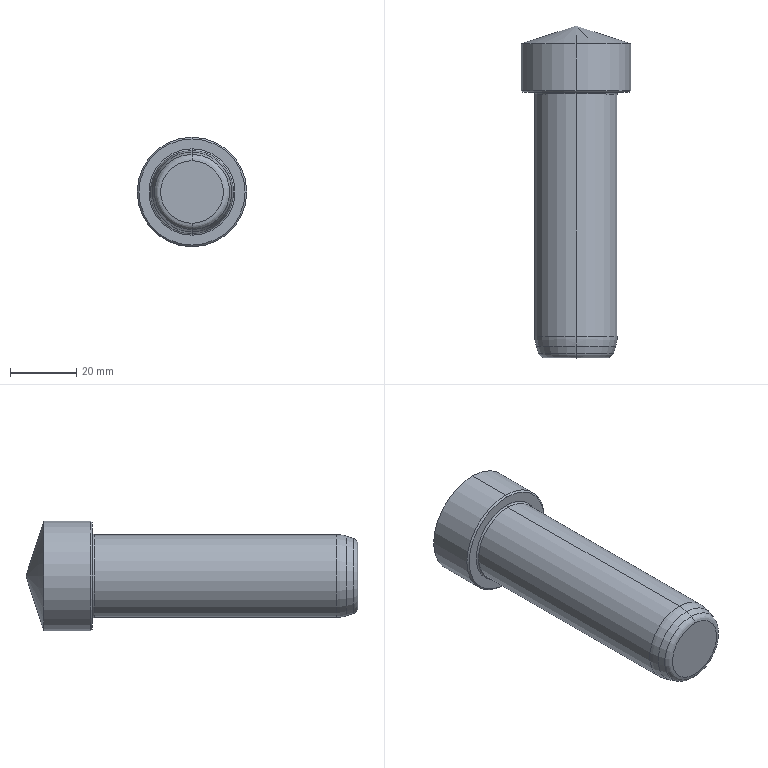Part | STEP file | Pino came 1 - Torre - 1 cav | 1 solid | 18 faces | box 33 x 100 x 33 mm | volume 52969 mm3 | cone 6 | torus 4 | cylinder 4 | other 2 | plane 2 | commonest cylinder face diameters 25 x2 33 x2
STEP:
#1=CARTESIAN_POINT('',(0.,0.,0.));
#2=DIRECTION('',(0.,0.,1.));
#3=DIRECTION('',(1.,0.,0.));
#4=AXIS2_PLACEMENT_3D('',#1,#2,#3);
#5=CARTESIAN_POINT('',(0.,0.,9.422));
#6=VERTEX_POINT('',#5);
#7=CARTESIAN_POINT('',(0.,0.,-9.422));
#8=VERTEX_POINT('',#7);
#9=CARTESIAN_POINT('',(0.,0.,0.));
#10=DIRECTION('',(0.,1.,0.));
#11=DIRECTION('',(0.,0.,1.));
#12=AXIS2_PLACEMENT_3D('',#9,#10,#11);
#13=CIRCLE('',#12,9.422);
#14=CARTESIAN_POINT('',(0.,2.,0.));
#15=DIRECTION('',(0.,1.,0.));
#16=DIRECTION('',(0.,0.,1.));
#17=AXIS2_PLACEMENT_3D('',#14,#15,#16);
#18=TOROIDAL_SURFACE('',#17,9.422,2.);
#19=CARTESIAN_POINT('',(0.,4.712));
#20=DIRECTION('',(1.,0.));
#21=VECTOR('',#20,1.);
#22=LINE('',#19,#21);
#23=(GEOMETRIC_REPRESENTATION_CONTEXT(2)PARAMETRIC_REPRESENTATION_CONTEXT()REPRESENTATION_CONTEXT('',''));
#24=DEFINITIONAL_REPRESENTATION('',(#22),#23);
#25=PCURVE('',#18,#24);
#26=CARTESIAN_POINT('',(0.,0.,0.));
#27=DIRECTION('',(0.,1.,0.));
#28=DIRECTION('',(0.,0.,1.));
#29=AXIS2_PLACEMENT_3D('',#26,#27,#28);
#30=PLANE('',#29);
#31=CARTESIAN_POINT('',(0.,0.));
#32=DIRECTION('',(1.,0.));
#33=AXIS2_PLACEMENT_2D('',#31,#32);
#34=CIRCLE('',#33,9.422);
#35=(GEOMETRIC_REPRESENTATION_CONTEXT(2)PARAMETRIC_REPRESENTATION_CONTEXT()REPRESENTATION_CONTEXT('',''));
#36=DEFINITIONAL_REPRESENTATION('',(#34),#35);
#37=PCURVE('',#30,#36);
#38=SURFACE_CURVE('',#13,(#25,#37),.PCURVE_S1.);
#39=EDGE_CURVE('',#6,#8,#38,.T.);
#40=ORIENTED_EDGE('',*,*,#39,.T.);
#41=CARTESIAN_POINT('',(0.,1.382,-11.324));
#42=VERTEX_POINT('',#41);
#43=CARTESIAN_POINT('',(0.,2.,-9.422));
#44=DIRECTION('',(1.,0.,0.));
#45=DIRECTION('',(0.,0.,-1.));
#46=AXIS2_PLACEMENT_3D('',#43,#44,#45);
#47=CIRCLE('',#46,2.);
#48=CARTESIAN_POINT('',(3.142,0.));
#49=DIRECTION('',(0.,1.));
#50=VECTOR('',#49,1.);
#51=LINE('',#48,#50);
#52=(GEOMETRIC_REPRESENTATION_CONTEXT(2)PARAMETRIC_REPRESENTATION_CONTEXT()REPRESENTATION_CONTEXT('',''));
#53=DEFINITIONAL_REPRESENTATION('',(#51),#52);
#54=PCURVE('',#18,#53);
#55=CARTESIAN_POINT('',(0.,2.,0.));
#56=DIRECTION('',(0.,1.,0.));
#57=DIRECTION('',(0.,0.,1.));
#58=AXIS2_PLACEMENT_3D('',#55,#56,#57);
#59=TOROIDAL_SURFACE('',#58,9.422,2.);
#60=CARTESIAN_POINT('',(3.142,0.));
#61=DIRECTION('',(0.,1.));
#62=VECTOR('',#61,1.);
#63=LINE('',#60,#62);
#64=(GEOMETRIC_REPRESENTATION_CONTEXT(2)PARAMETRIC_REPRESENTATION_CONTEXT()REPRESENTATION_CONTEXT('',''));
#65=DEFINITIONAL_REPRESENTATION('',(#63),#64);
#66=PCURVE('',#59,#65);
#67=SURFACE_CURVE('',#47,(#54,#66),.PCURVE_S1.);
#68=EDGE_CURVE('',#8,#42,#67,.T.);
#69=ORIENTED_EDGE('',*,*,#68,.T.);
#70=CARTESIAN_POINT('',(0.,1.382,11.324));
#71=VERTEX_POINT('',#70);
#72=CARTESIAN_POINT('',(0.,1.382,0.));
#73=DIRECTION('',(0.,1.,0.));
#74=DIRECTION('',(0.,0.,1.));
#75=AXIS2_PLACEMENT_3D('',#72,#73,#74);
#76=CIRCLE('',#75,11.324);
#77=CARTESIAN_POINT('',(0.,5.969));
#78=DIRECTION('',(1.,0.));
#79=VECTOR('',#78,1.);
#80=LINE('',#77,#79);
#81=(GEOMETRIC_REPRESENTATION_CONTEXT(2)PARAMETRIC_REPRESENTATION_CONTEXT()REPRESENTATION_CONTEXT('',''));
#82=DEFINITIONAL_REPRESENTATION('',(#80),#81);
#83=PCURVE('',#18,#82);
#84=CARTESIAN_POINT('',(0.,1.382,0.));
#85=DIRECTION('',(0.,1.,0.));
#86=DIRECTION('',(0.,0.,1.));
#87=AXIS2_PLACEMENT_3D('',#84,#85,#86);
#88=CONICAL_SURFACE('',#87,11.324,0.3142);
#89=CARTESIAN_POINT('',(0.,0.));
#90=DIRECTION('',(1.,0.));
#91=VECTOR('',#90,1.);
#92=LINE('',#89,#91);
#93=(GEOMETRIC_REPRESENTATION_CONTEXT(2)PARAMETRIC_REPRESENTATION_CONTEXT()REPRESENTATION_CONTEXT('',''));
#94=DEFINITIONAL_REPRESENTATION('',(#92),#93);
#95=PCURVE('',#88,#94);
#96=SURFACE_CURVE('',#76,(#83,#95),.PCURVE_S1.);
#97=EDGE_CURVE('',#71,#42,#96,.T.);
#98=ORIENTED_EDGE('',*,*,#97,.F.);
#99=CARTESIAN_POINT('',(0.,2.,9.422));
#100=DIRECTION('',(-1.,0.,0.));
#101=DIRECTION('',(0.,0.,1.));
#102=AXIS2_PLACEMENT_3D('',#99,#100,#101);
#103=CIRCLE('',#102,2.);
#104=CARTESIAN_POINT('',(0.,0.));
#105=DIRECTION('',(0.,1.));
#106=VECTOR('',#105,1.);
#107=LINE('',#104,#106);
#108=(GEOMETRIC_REPRESENTATION_CONTEXT(2)PARAMETRIC_REPRESENTATION_CONTEXT()REPRESENTATION_CONTEXT('',''));
#109=DEFINITIONAL_REPRESENTATION('',(#107),#108);
#110=PCURVE('',#18,#109);
#111=CARTESIAN_POINT('',(6.283,0.));
#112=DIRECTION('',(0.,1.));
#113=VECTOR('',#112,1.);
#114=LINE('',#111,#113);
#115=(GEOMETRIC_REPRESENTATION_CONTEXT(2)PARAMETRIC_REPRESENTATION_CONTEXT()REPRESENTATION_CONTEXT('',''));
#116=DEFINITIONAL_REPRESENTATION('',(#114),#115);
#117=PCURVE('',#59,#116);
#118=SURFACE_CURVE('',#103,(#110,#117),.PCURVE_S1.);
#119=EDGE_CURVE('',#6,#71,#118,.T.);
#120=ORIENTED_EDGE('',*,*,#119,.F.);
#121=EDGE_LOOP('',(#40,#69,#98,#120));
#122=FACE_BOUND('',#121,.T.);
#123=ADVANCED_FACE('',(#122),#18,.T.);
#124=ORIENTED_EDGE('',*,*,#97,.T.);
#125=CARTESIAN_POINT('',(0.,3.494,-12.011));
#126=VERTEX_POINT('',#125);
#127=CARTESIAN_POINT('',(0.,1.382,-11.324));
#128=DIRECTION('',(0.,0.9511,-0.309));
#129=VECTOR('',#128,1.);
#130=LINE('',#127,#129);
#131=CARTESIAN_POINT('',(3.142,0.));
#132=DIRECTION('',(0.,1.));
#133=VECTOR('',#132,1.);
#134=LINE('',#131,#133);
#135=(GEOMETRIC_REPRESENTATION_CONTEXT(2)PARAMETRIC_REPRESENTATION_CONTEXT()REPRESENTATION_CONTEXT('',''));
#136=DEFINITIONAL_REPRESENTATION('',(#134),#135);
#137=PCURVE('',#88,#136);
#138=CARTESIAN_POINT('',(0.,1.382,0.));
#139=DIRECTION('',(0.,1.,0.));
#140=DIRECTION('',(0.,0.,1.));
#141=AXIS2_PLACEMENT_3D('',#138,#139,#140);
#142=CONICAL_SURFACE('',#141,11.324,0.3142);
#143=CARTESIAN_POINT('',(3.142,0.));
#144=DIRECTION('',(0.,1.));
#145=VECTOR('',#144,1.);
#146=LINE('',#143,#145);
#147=(GEOMETRIC_REPRESENTATION_CONTEXT(2)PARAMETRIC_REPRESENTATION_CONTEXT()REPRESENTATION_CONTEXT('',''));
#148=DEFINITIONAL_REPRESENTATION('',(#146),#147);
#149=PCURVE('',#142,#148);
#150=SURFACE_CURVE('',#130,(#137,#149),.PCURVE_S1.);
#151=EDGE_CURVE('',#42,#126,#150,.T.);
#152=ORIENTED_EDGE('',*,*,#151,.T.);
#153=CARTESIAN_POINT('',(0.,3.494,12.011));
#154=VERTEX_POINT('',#153);
#155=CARTESIAN_POINT('',(0.,3.494,0.));
#156=DIRECTION('',(0.,1.,0.));
#157=DIRECTION('',(0.,0.,1.));
#158=AXIS2_PLACEMENT_3D('',#155,#156,#157);
#159=CIRCLE('',#158,12.011);
#160=CARTESIAN_POINT('',(0.,2.112));
#161=DIRECTION('',(1.,0.));
#162=VECTOR('',#161,1.);
#163=LINE('',#160,#162);
#164=(GEOMETRIC_REPRESENTATION_CONTEXT(2)PARAMETRIC_REPRESENTATION_CONTEXT()REPRESENTATION_CONTEXT('',''));
#165=DEFINITIONAL_REPRESENTATION('',(#163),#164);
#166=PCURVE('',#88,#165);
#167=CARTESIAN_POINT('',(0.,3.494,12.011));
#168=CARTESIAN_POINT('',(0.,4.091,12.205));
#169=CARTESIAN_POINT('',(0.,4.704,12.352));
#170=CARTESIAN_POINT('',(0.,5.327,12.451));
#171=CARTESIAN_POINT('',(0.,5.956,12.5));
#172=CARTESIAN_POINT('',(0.,6.584,12.5));
#173=B_SPLINE_CURVE_WITH_KNOTS('',5,(#167,#168,#169,#170,#171,#172),.UNSPECIFIED.,.F.,.F.,(6,6),(5.969,6.283),.PIECEWISE_BEZIER_KNOTS.);
#174=CARTESIAN_POINT('',(0.,6.584,0.));
#175=DIRECTION('',(0.,1.,0.));
#176=AXIS1_PLACEMENT('',#174,#175);
#177=SURFACE_OF_REVOLUTION('',#173,#176);
#178=CARTESIAN_POINT('',(0.,5.969));
#179=DIRECTION('',(1.,0.));
#180=VECTOR('',#179,1.);
#181=LINE('',#178,#180);
#182=(GEOMETRIC_REPRESENTATION_CONTEXT(2)PARAMETRIC_REPRESENTATION_CONTEXT()REPRESENTATION_CONTEXT('',''));
#183=DEFINITIONAL_REPRESENTATION('',(#181),#182);
#184=PCURVE('',#177,#183);
#185=SURFACE_CURVE('',#159,(#166,#184),.PCURVE_S1.);
#186=EDGE_CURVE('',#154,#126,#185,.T.);
#187=ORIENTED_EDGE('',*,*,#186,.F.);
#188=CARTESIAN_POINT('',(0.,1.382,11.324));
#189=DIRECTION('',(0.,0.9511,0.309));
#190=VECTOR('',#189,1.);
#191=LINE('',#188,#190);
#192=CARTESIAN_POINT('',(0.,0.));
#193=DIRECTION('',(0.,1.));
#194=VECTOR('',#193,1.);
#195=LINE('',#192,#194);
#196=(GEOMETRIC_REPRESENTATION_CONTEXT(2)PARAMETRIC_REPRESENTATION_CONTEXT()REPRESENTATION_CONTEXT('',''));
#197=DEFINITIONAL_REPRESENTATION('',(#195),#196);
#198=PCURVE('',#88,#197);
#199=CARTESIAN_POINT('',(6.283,0.));
#200=DIRECTION('',(0.,1.));
#201=VECTOR('',#200,1.);
#202=LINE('',#199,#201);
#203=(GEOMETRIC_REPRESENTATION_CONTEXT(2)PARAMETRIC_REPRESENTATION_CONTEXT()REPRESENTATION_CONTEXT('',''));
#204=DEFINITIONAL_REPRESENTATION('',(#202),#203);
#205=PCURVE('',#142,#204);
#206=SURFACE_CURVE('',#191,(#198,#205),.PCURVE_S1.);
#207=EDGE_CURVE('',#71,#154,#206,.T.);
#208=ORIENTED_EDGE('',*,*,#207,.F.);
#209=EDGE_LOOP('',(#124,#152,#187,#208));
#210=FACE_BOUND('',#209,.T.);
#211=ADVANCED_FACE('',(#210),#88,.T.);
#212=ORIENTED_EDGE('',*,*,#186,.T.);
#213=CARTESIAN_POINT('',(0.,6.584,-12.5));
#214=VERTEX_POINT('',#213);
#215=CARTESIAN_POINT('',(0.,6.584,-2.5));
#216=DIRECTION('',(1.,0.,0.));
#217=DIRECTION('',(0.,0.,-1.));
#218=AXIS2_PLACEMENT_3D('',#215,#216,#217);
#219=CIRCLE('',#218,10.);
#220=CARTESIAN_POINT('',(3.142,0.));
#221=DIRECTION('',(0.,1.));
#222=VECTOR('',#221,1.);
#223=LINE('',#220,#222);
#224=(GEOMETRIC_REPRESENTATION_CONTEXT(2)PARAMETRIC_REPRESENTATION_CONTEXT()REPRESENTATION_CONTEXT('',''));
#225=DEFINITIONAL_REPRESENTATION('',(#223),#224);
#226=PCURVE('',#177,#225);
#227=CARTESIAN_POINT('',(0.,3.494,12.011));
#228=CARTESIAN_POINT('',(0.,4.091,12.205));
#229=CARTESIAN_POINT('',(0.,4.704,12.352));
#230=CARTESIAN_POINT('',(0.,5.327,12.451));
#231=CARTESIAN_POINT('',(0.,5.956,12.5));
#232=CARTESIAN_POINT('',(0.,6.584,12.5));
#233=B_SPLINE_CURVE_WITH_KNOTS('',5,(#227,#228,#229,#230,#231,#232),.UNSPECIFIED.,.F.,.F.,(6,6),(5.969,6.283),.PIECEWISE_BEZIER_KNOTS.);
#234=CARTESIAN_POINT('',(0.,6.584,0.));
#235=DIRECTION('',(0.,1.,0.));
#236=AXIS1_PLACEMENT('',#234,#235);
#237=SURFACE_OF_REVOLUTION('',#233,#236);
#238=CARTESIAN_POINT('',(3.142,0.));
#239=DIRECTION('',(0.,1.));
#240=VECTOR('',#239,1.);
#241=LINE('',#238,#240);
#242=(GEOMETRIC_REPRESENTATION_CONTEXT(2)PARAMETRIC_REPRESENTATION_CONTEXT()REPRESENTATION_CONTEXT('',''));
#243=DEFINITIONAL_REPRESENTATION('',(#241),#242);
#244=PCURVE('',#237,#243);
#245=SURFACE_CURVE('',#219,(#226,#244),.PCURVE_S1.);
#246=EDGE_CURVE('',#126,#214,#245,.T.);
#247=ORIENTED_EDGE('',*,*,#246,.T.);
#248=CARTESIAN_POINT('',(0.,6.584,12.5));
#249=VERTEX_POINT('',#248);
#250=CARTESIAN_POINT('',(0.,6.584,0.));
#251=DIRECTION('',(0.,1.,0.));
#252=DIRECTION('',(0.,0.,1.));
#253=AXIS2_PLACEMENT_3D('',#250,#251,#252);
#254=CIRCLE('',#253,12.5);
#255=CARTESIAN_POINT('',(0.,6.283));
#256=DIRECTION('',(1.,0.));
#257=VECTOR('',#256,1.);
#258=LINE('',#255,#257);
#259=(GEOMETRIC_REPRESENTATION_CONTEXT(2)PARAMETRIC_REPRESENTATION_CONTEXT()REPRESENTATION_CONTEXT('',''));
#260=DEFINITIONAL_REPRESENTATION('',(#258),#259);
#261=PCURVE('',#177,#260);
#262=CARTESIAN_POINT('',(0.,100.,0.));
#263=DIRECTION('',(0.,1.,0.));
#264=DIRECTION('',(0.,0.,1.));
#265=AXIS2_PLACEMENT_3D('',#262,#263,#264);
#266=CYLINDRICAL_SURFACE('',#265,12.5);
#267=CARTESIAN_POINT('',(0.,-93.416));
#268=DIRECTION('',(1.,0.));
#269=VECTOR('',#268,1.);
#270=LINE('',#267,#269);
#271=(GEOMETRIC_REPRESENTATION_CONTEXT(2)PARAMETRIC_REPRESENTATION_CONTEXT()REPRESENTATION_CONTEXT('',''));
#272=DEFINITIONAL_REPRESENTATION('',(#270),#271);
#273=PCURVE('',#266,#272);
#274=SURFACE_CURVE('',#254,(#261,#273),.PCURVE_S1.);
#275=EDGE_CURVE('',#249,#214,#274,.T.);
#276=ORIENTED_EDGE('',*,*,#275,.F.);
#277=CARTESIAN_POINT('',(0.,6.584,2.5));
#278=DIRECTION('',(-1.,0.,0.));
#279=DIRECTION('',(0.,0.,1.));
#280=AXIS2_PLACEMENT_3D('',#277,#278,#279);
#281=CIRCLE('',#280,10.);
#282=CARTESIAN_POINT('',(0.,0.));
#283=DIRECTION('',(0.,1.));
#284=VECTOR('',#283,1.);
#285=LINE('',#282,#284);
#286=(GEOMETRIC_REPRESENTATION_CONTEXT(2)PARAMETRIC_REPRESENTATION_CONTEXT()REPRESENTATION_CONTEXT('',''));
#287=DEFINITIONAL_REPRESENTATION('',(#285),#286);
#288=PCURVE('',#177,#287);
#289=CARTESIAN_POINT('',(6.283,0.));
#290=DIRECTION('',(0.,1.));
#291=VECTOR('',#290,1.);
#292=LINE('',#289,#291);
#293=(GEOMETRIC_REPRESENTATION_CONTEXT(2)PARAMETRIC_REPRESENTATION_CONTEXT()REPRESENTATION_CONTEXT('',''));
#294=DEFINITIONAL_REPRESENTATION('',(#292),#293);
#295=PCURVE('',#237,#294);
#296=SURFACE_CURVE('',#281,(#288,#295),.PCURVE_S1.);
#297=EDGE_CURVE('',#154,#249,#296,.T.);
#298=ORIENTED_EDGE('',*,*,#297,.F.);
#299=EDGE_LOOP('',(#212,#247,#276,#298));
#300=FACE_BOUND('',#299,.T.);
#301=ADVANCED_FACE('',(#300),#177,.T.);
#302=ORIENTED_EDGE('',*,*,#275,.T.);
#303=CARTESIAN_POINT('',(0.,79.5,-12.5));
#304=VERTEX_POINT('',#303);
#305=CARTESIAN_POINT('',(0.,100.,-12.5));
#306=DIRECTION('',(0.,1.,0.));
#307=VECTOR('',#306,1.);
#308=LINE('',#305,#307);
#309=CARTESIAN_POINT('',(3.142,0.));
#310=DIRECTION('',(0.,1.));
#311=VECTOR('',#310,1.);
#312=LINE('',#309,#311);
#313=(GEOMETRIC_REPRESENTATION_CONTEXT(2)PARAMETRIC_REPRESENTATION_CONTEXT()REPRESENTATION_CONTEXT('',''));
#314=DEFINITIONAL_REPRESENTATION('',(#312),#313);
#315=PCURVE('',#266,#314);
#316=CARTESIAN_POINT('',(0.,100.,0.));
#317=DIRECTION('',(0.,1.,0.));
#318=DIRECTION('',(0.,0.,1.));
#319=AXIS2_PLACEMENT_3D('',#316,#317,#318);
#320=CYLINDRICAL_SURFACE('',#319,12.5);
#321=CARTESIAN_POINT('',(3.142,0.));
#322=DIRECTION('',(0.,1.));
#323=VECTOR('',#322,1.);
#324=LINE('',#321,#323);
#325=(GEOMETRIC_REPRESENTATION_CONTEXT(2)PARAMETRIC_REPRESENTATION_CONTEXT()REPRESENTATION_CONTEXT('',''));
#326=DEFINITIONAL_REPRESENTATION('',(#324),#325);
#327=PCURVE('',#320,#326);
#328=SURFACE_CURVE('',#308,(#315,#327),.PCURVE_S1.);
#329=EDGE_CURVE('',#214,#304,#328,.T.);
#330=ORIENTED_EDGE('',*,*,#329,.T.);
#331=CARTESIAN_POINT('',(0.,79.5,12.5));
#332=VERTEX_POINT('',#331);
#333=CARTESIAN_POINT('',(0.,79.5,0.));
#334=DIRECTION('',(0.,1.,0.));
#335=DIRECTION('',(0.,0.,1.));
#336=AXIS2_PLACEMENT_3D('',#333,#334,#335);
#337=CIRCLE('',#336,12.5);
#338=CARTESIAN_POINT('',(0.,-20.5));
#339=DIRECTION('',(1.,0.));
#340=VECTOR('',#339,1.);
#341=LINE('',#338,#340);
#342=(GEOMETRIC_REPRESENTATION_CONTEXT(2)PARAMETRIC_REPRESENTATION_CONTEXT()REPRESENTATION_CONTEXT('',''));
#343=DEFINITIONAL_REPRESENTATION('',(#341),#342);
#344=PCURVE('',#266,#343);
#345=CARTESIAN_POINT('',(0.,79.5,0.));
#346=DIRECTION('',(0.,1.,0.));
#347=DIRECTION('',(0.,0.,1.));
#348=AXIS2_PLACEMENT_3D('',#345,#346,#347);
#349=TOROIDAL_SURFACE('',#348,13.,0.5);
#350=CARTESIAN_POINT('',(0.,3.142));
#351=DIRECTION('',(1.,0.));
#352=VECTOR('',#351,1.);
#353=LINE('',#350,#352);
#354=(GEOMETRIC_REPRESENTATION_CONTEXT(2)PARAMETRIC_REPRESENTATION_CONTEXT()REPRESENTATION_CONTEXT('',''));
#355=DEFINITIONAL_REPRESENTATION('',(#353),#354);
#356=PCURVE('',#349,#355);
#357=SURFACE_CURVE('',#337,(#344,#356),.PCURVE_S1.);
#358=EDGE_CURVE('',#332,#304,#357,.T.);
#359=ORIENTED_EDGE('',*,*,#358,.F.);
#360=CARTESIAN_POINT('',(0.,100.,12.5));
#361=DIRECTION('',(0.,1.,0.));
#362=VECTOR('',#361,1.);
#363=LINE('',#360,#362);
#364=CARTESIAN_POINT('',(0.,0.));
#365=DIRECTION('',(0.,1.));
#366=VECTOR('',#365,1.);
#367=LINE('',#364,#366);
#368=(GEOMETRIC_REPRESENTATION_CONTEXT(2)PARAMETRIC_REPRESENTATION_CONTEXT()REPRESENTATION_CONTEXT('',''));
#369=DEFINITIONAL_REPRESENTATION('',(#367),#368);
#370=PCURVE('',#266,#369);
#371=CARTESIAN_POINT('',(6.283,0.));
#372=DIRECTION('',(0.,1.));
#373=VECTOR('',#372,1.);
#374=LINE('',#371,#373);
#375=(GEOMETRIC_REPRESENTATION_CONTEXT(2)PARAMETRIC_REPRESENTATION_CONTEXT()REPRESENTATION_CONTEXT('',''));
#376=DEFINITIONAL_REPRESENTATION('',(#374),#375);
#377=PCURVE('',#320,#376);
#378=SURFACE_CURVE('',#363,(#370,#377),.PCURVE_S1.);
#379=EDGE_CURVE('',#249,#332,#378,.T.);
#380=ORIENTED_EDGE('',*,*,#379,.F.);
#381=EDGE_LOOP('',(#302,#330,#359,#380));
#382=FACE_BOUND('',#381,.T.);
#383=ADVANCED_FACE('',(#382),#266,.T.);
#384=CARTESIAN_POINT('',(0.,80.,13.));
#385=VERTEX_POINT('',#384);
#386=CARTESIAN_POINT('',(0.,79.5,13.));
#387=DIRECTION('',(-1.,0.,0.));
#388=DIRECTION('',(0.,0.,1.));
#389=AXIS2_PLACEMENT_3D('',#386,#387,#388);
#390=CIRCLE('',#389,0.5);
#391=CARTESIAN_POINT('',(0.,79.5,0.));
#392=DIRECTION('',(0.,1.,0.));
#393=DIRECTION('',(0.,0.,1.));
#394=AXIS2_PLACEMENT_3D('',#391,#392,#393);
#395=TOROIDAL_SURFACE('',#394,13.,0.5);
#396=CARTESIAN_POINT('',(6.283,0.));
#397=DIRECTION('',(0.,1.));
#398=VECTOR('',#397,1.);
#399=LINE('',#396,#398);
#400=(GEOMETRIC_REPRESENTATION_CONTEXT(2)PARAMETRIC_REPRESENTATION_CONTEXT()REPRESENTATION_CONTEXT('',''));
#401=DEFINITIONAL_REPRESENTATION('',(#399),#400);
#402=PCURVE('',#395,#401);
#403=CARTESIAN_POINT('',(0.,0.));
#404=DIRECTION('',(0.,1.));
#405=VECTOR('',#404,1.);
#406=LINE('',#403,#405);
#407=(GEOMETRIC_REPRESENTATION_CONTEXT(2)PARAMETRIC_REPRESENTATION_CONTEXT()REPRESENTATION_CONTEXT('',''));
#408=DEFINITIONAL_REPRESENTATION('',(#406),#407);
#409=PCURVE('',#349,#408);
#410=SURFACE_CURVE('',#390,(#402,#409),.PCURVE_S1.);
#411=EDGE_CURVE('',#385,#332,#410,.T.);
#412=ORIENTED_EDGE('',*,*,#411,.T.);
#413=CARTESIAN_POINT('',(0.,79.5,0.));
#414=DIRECTION('',(0.,1.,0.));
#415=DIRECTION('',(0.,0.,1.));
#416=AXIS2_PLACEMENT_3D('',#413,#414,#415);
#417=CIRCLE('',#416,12.5);
#418=CARTESIAN_POINT('',(0.,3.142));
#419=DIRECTION('',(1.,0.));
#420=VECTOR('',#419,1.);
#421=LINE('',#418,#420);
#422=(GEOMETRIC_REPRESENTATION_CONTEXT(2)PARAMETRIC_REPRESENTATION_CONTEXT()REPRESENTATION_CONTEXT('',''));
#423=DEFINITIONAL_REPRESENTATION('',(#421),#422);
#424=PCURVE('',#395,#423);
#425=CARTESIAN_POINT('',(0.,-20.5));
#426=DIRECTION('',(1.,0.));
#427=VECTOR('',#426,1.);
#428=LINE('',#425,#427);
#429=(GEOMETRIC_REPRESENTATION_CONTEXT(2)PARAMETRIC_REPRESENTATION_CONTEXT()REPRESENTATION_CONTEXT('',''));
#430=DEFINITIONAL_REPRESENTATION('',(#428),#429);
#431=PCURVE('',#320,#430);
#432=SURFACE_CURVE('',#417,(#424,#431),.PCURVE_S1.);
#433=EDGE_CURVE('',#304,#332,#432,.T.);
#434=ORIENTED_EDGE('',*,*,#433,.F.);
#435=CARTESIAN_POINT('',(0.,80.,-13.));
#436=VERTEX_POINT('',#435);
#437=CARTESIAN_POINT('',(0.,79.5,-13.));
#438=DIRECTION('',(1.,0.,0.));
#439=DIRECTION('',(0.,0.,-1.));
#440=AXIS2_PLACEMENT_3D('',#437,#438,#439);
#441=CIRCLE('',#440,0.5);
#442=CARTESIAN_POINT('',(3.142,0.));
#443=DIRECTION('',(0.,1.));
#444=VECTOR('',#443,1.);
#445=LINE('',#442,#444);
#446=(GEOMETRIC_REPRESENTATION_CONTEXT(2)PARAMETRIC_REPRESENTATION_CONTEXT()REPRESENTATION_CONTEXT('',''));
#447=DEFINITIONAL_REPRESENTATION('',(#445),#446);
#448=PCURVE('',#395,#447);
#449=CARTESIAN_POINT('',(3.142,0.));
#450=DIRECTION('',(0.,1.));
#451=VECTOR('',#450,1.);
#452=LINE('',#449,#451);
#453=(GEOMETRIC_REPRESENTATION_CONTEXT(2)PARAMETRIC_REPRESENTATION_CONTEXT()REPRESENTATION_CONTEXT('',''));
#454=DEFINITIONAL_REPRESENTATION('',(#452),#453);
#455=PCURVE('',#349,#454);
#456=SURFACE_CURVE('',#441,(#448,#455),.PCURVE_S1.);
#457=EDGE_CURVE('',#436,#304,#456,.T.);
#458=ORIENTED_EDGE('',*,*,#457,.F.);
#459=CARTESIAN_POINT('',(0.,80.,0.));
#460=DIRECTION('',(0.,1.,0.));
#461=DIRECTION('',(0.,0.,1.));
#462=AXIS2_PLACEMENT_3D('',#459,#460,#461);
#463=CIRCLE('',#462,13.);
#464=CARTESIAN_POINT('',(0.,1.571));
#465=DIRECTION('',(1.,0.));
#466=VECTOR('',#465,1.);
#467=LINE('',#464,#466);
#468=(GEOMETRIC_REPRESENTATION_CONTEXT(2)PARAMETRIC_REPRESENTATION_CONTEXT()REPRESENTATION_CONTEXT('',''));
#469=DEFINITIONAL_REPRESENTATION('',(#467),#468);
#470=PCURVE('',#395,#469);
#471=CARTESIAN_POINT('',(0.,80.,-13.));
#472=DIRECTION('',(0.,1.,0.));
#473=DIRECTION('',(0.,0.,1.));
#474=AXIS2_PLACEMENT_3D('',#471,#472,#473);
#475=PLANE('',#474);
#476=CARTESIAN_POINT('',(13.,0.));
#477=DIRECTION('',(1.,0.));
#478=AXIS2_PLACEMENT_2D('',#476,#477);
#479=CIRCLE('',#478,13.);
#480=(GEOMETRIC_REPRESENTATION_CONTEXT(2)PARAMETRIC_REPRESENTATION_CONTEXT()REPRESENTATION_CONTEXT('',''));
#481=DEFINITIONAL_REPRESENTATION('',(#479),#480);
#482=PCURVE('',#475,#481);
#483=SURFACE_CURVE('',#463,(#470,#482),.PCURVE_S1.);
#484=EDGE_CURVE('',#436,#385,#483,.T.);
#485=ORIENTED_EDGE('',*,*,#484,.T.);
#486=EDGE_LOOP('',(#412,#434,#458,#485));
#487=FACE_BOUND('',#486,.F.);
#488=ADVANCED_FACE('',(#487),#395,.F.);
#489=CARTESIAN_POINT('',(0.,80.,16.));
#490=VERTEX_POINT('',#489);
#491=CARTESIAN_POINT('',(0.,80.,-16.));
#492=VERTEX_POINT('',#491);
#493=CARTESIAN_POINT('',(0.,80.,0.));
#494=DIRECTION('',(0.,1.,0.));
#495=DIRECTION('',(0.,0.,1.));
#496=AXIS2_PLACEMENT_3D('',#493,#494,#495);
#497=CIRCLE('',#496,16.);
#498=CARTESIAN_POINT('',(0.,80.,0.));
#499=DIRECTION('',(0.,1.,0.));
#500=DIRECTION('',(0.,0.,1.));
#501=AXIS2_PLACEMENT_3D('',#498,#499,#500);
#502=CONICAL_SURFACE('',#501,16.,0.7854);
#503=CARTESIAN_POINT('',(0.,0.));
#504=DIRECTION('',(1.,0.));
#505=VECTOR('',#504,1.);
#506=LINE('',#503,#505);
#507=(GEOMETRIC_REPRESENTATION_CONTEXT(2)PARAMETRIC_REPRESENTATION_CONTEXT()REPRESENTATION_CONTEXT('',''));
#508=DEFINITIONAL_REPRESENTATION('',(#506),#507);
#509=PCURVE('',#502,#508);
#510=CARTESIAN_POINT('',(13.,0.));
#511=DIRECTION('',(1.,0.));
#512=AXIS2_PLACEMENT_2D('',#510,#511);
#513=CIRCLE('',#512,16.);
#514=(GEOMETRIC_REPRESENTATION_CONTEXT(2)PARAMETRIC_REPRESENTATION_CONTEXT()REPRESENTATION_CONTEXT('',''));
#515=DEFINITIONAL_REPRESENTATION('',(#513),#514);
#516=PCURVE('',#475,#515);
#517=SURFACE_CURVE('',#497,(#509,#516),.PCURVE_S1.);
#518=EDGE_CURVE('',#490,#492,#517,.T.);
#519=ORIENTED_EDGE('',*,*,#518,.T.);
#520=CARTESIAN_POINT('',(0.,80.5,-16.5));
#521=VERTEX_POINT('',#520);
#522=CARTESIAN_POINT('',(0.,80.,-16.));
#523=DIRECTION('',(0.,0.7071,-0.7071));
#524=VECTOR('',#523,1.);
#525=LINE('',#522,#524);
#526=CARTESIAN_POINT('',(3.142,0.));
#527=DIRECTION('',(0.,1.));
#528=VECTOR('',#527,1.);
#529=LINE('',#526,#528);
#530=(GEOMETRIC_REPRESENTATION_CONTEXT(2)PARAMETRIC_REPRESENTATION_CONTEXT()REPRESENTATION_CONTEXT('',''));
#531=DEFINITIONAL_REPRESENTATION('',(#529),#530);
#532=PCURVE('',#502,#531);
#533=CARTESIAN_POINT('',(0.,80.,0.));
#534=DIRECTION('',(0.,1.,0.));
#535=DIRECTION('',(0.,0.,1.));
#536=AXIS2_PLACEMENT_3D('',#533,#534,#535);
#537=CONICAL_SURFACE('',#536,16.,0.7854);
#538=CARTESIAN_POINT('',(3.142,0.));
#539=DIRECTION('',(0.,1.));
#540=VECTOR('',#539,1.);
#541=LINE('',#538,#540);
#542=(GEOMETRIC_REPRESENTATION_CONTEXT(2)PARAMETRIC_REPRESENTATION_CONTEXT()REPRESENTATION_CONTEXT('',''));
#543=DEFINITIONAL_REPRESENTATION('',(#541),#542);
#544=PCURVE('',#537,#543);
#545=SURFACE_CURVE('',#525,(#532,#544),.PCURVE_S1.);
#546=EDGE_CURVE('',#492,#521,#545,.T.);
#547=ORIENTED_EDGE('',*,*,#546,.T.);
#548=CARTESIAN_POINT('',(0.,80.5,16.5));
#549=VERTEX_POINT('',#548);
#550=CARTESIAN_POINT('',(0.,80.5,0.));
#551=DIRECTION('',(0.,1.,0.));
#552=DIRECTION('',(0.,0.,1.));
#553=AXIS2_PLACEMENT_3D('',#550,#551,#552);
#554=CIRCLE('',#553,16.5);
#555=CARTESIAN_POINT('',(0.,0.5));
#556=DIRECTION('',(1.,0.));
#557=VECTOR('',#556,1.);
#558=LINE('',#555,#557);
#559=(GEOMETRIC_REPRESENTATION_CONTEXT(2)PARAMETRIC_REPRESENTATION_CONTEXT()REPRESENTATION_CONTEXT('',''));
#560=DEFINITIONAL_REPRESENTATION('',(#558),#559);
#561=PCURVE('',#502,#560);
#562=CARTESIAN_POINT('',(0.,100.,0.));
#563=DIRECTION('',(0.,1.,0.));
#564=DIRECTION('',(0.,0.,1.));
#565=AXIS2_PLACEMENT_3D('',#562,#563,#564);
#566=CYLINDRICAL_SURFACE('',#565,16.5);
#567=CARTESIAN_POINT('',(0.,-19.5));
#568=DIRECTION('',(1.,0.));
#569=VECTOR('',#568,1.);
#570=LINE('',#567,#569);
#571=(GEOMETRIC_REPRESENTATION_CONTEXT(2)PARAMETRIC_REPRESENTATION_CONTEXT()REPRESENTATION_CONTEXT('',''));
#572=DEFINITIONAL_REPRESENTATION('',(#570),#571);
#573=PCURVE('',#566,#572);
#574=SURFACE_CURVE('',#554,(#561,#573),.PCURVE_S1.);
#575=EDGE_CURVE('',#549,#521,#574,.T.);
#576=ORIENTED_EDGE('',*,*,#575,.F.);
#577=CARTESIAN_POINT('',(0.,80.,16.));
#578=DIRECTION('',(0.,0.7071,0.7071));
#579=VECTOR('',#578,1.);
#580=LINE('',#577,#579);
#581=CARTESIAN_POINT('',(0.,0.));
#582=DIRECTION('',(0.,1.));
#583=VECTOR('',#582,1.);
#584=LINE('',#581,#583);
#585=(GEOMETRIC_REPRESENTATION_CONTEXT(2)PARAMETRIC_REPRESENTATION_CONTEXT()REPRESENTATION_CONTEXT('',''));
#586=DEFINITIONAL_REPRESENTATION('',(#584),#585);
#587=PCURVE('',#502,#586);
#588=CARTESIAN_POINT('',(6.283,0.));
#589=DIRECTION('',(0.,1.));
#590=VECTOR('',#589,1.);
#591=LINE('',#588,#590);
#592=(GEOMETRIC_REPRESENTATION_CONTEXT(2)PARAMETRIC_REPRESENTATION_CONTEXT()REPRESENTATION_CONTEXT('',''));
#593=DEFINITIONAL_REPRESENTATION('',(#591),#592);
#594=PCURVE('',#537,#593);
#595=SURFACE_CURVE('',#580,(#587,#594),.PCURVE_S1.);
#596=EDGE_CURVE('',#490,#549,#595,.T.);
#597=ORIENTED_EDGE('',*,*,#596,.F.);
#598=EDGE_LOOP('',(#519,#547,#576,#597));
#599=FACE_BOUND('',#598,.T.);
#600=ADVANCED_FACE('',(#599),#502,.T.);
#601=ORIENTED_EDGE('',*,*,#575,.T.);
#602=CARTESIAN_POINT('',(0.,94.639,-16.5));
#603=VERTEX_POINT('',#602);
#604=CARTESIAN_POINT('',(0.,100.,-16.5));
#605=DIRECTION('',(0.,1.,0.));
#606=VECTOR('',#605,1.);
#607=LINE('',#604,#606);
#608=CARTESIAN_POINT('',(3.142,0.));
#609=DIRECTION('',(0.,1.));
#610=VECTOR('',#609,1.);
#611=LINE('',#608,#610);
#612=(GEOMETRIC_REPRESENTATION_CONTEXT(2)PARAMETRIC_REPRESENTATION_CONTEXT()REPRESENTATION_CONTEXT('',''));
#613=DEFINITIONAL_REPRESENTATION('',(#611),#612);
#614=PCURVE('',#566,#613);
#615=CARTESIAN_POINT('',(0.,100.,0.));
#616=DIRECTION('',(0.,1.,0.));
#617=DIRECTION('',(0.,0.,1.));
#618=AXIS2_PLACEMENT_3D('',#615,#616,#617);
#619=CYLINDRICAL_SURFACE('',#618,16.5);
#620=CARTESIAN_POINT('',(3.142,0.));
#621=DIRECTION('',(0.,1.));
#622=VECTOR('',#621,1.);
#623=LINE('',#620,#622);
#624=(GEOMETRIC_REPRESENTATION_CONTEXT(2)PARAMETRIC_REPRESENTATION_CONTEXT()REPRESENTATION_CONTEXT('',''));
#625=DEFINITIONAL_REPRESENTATION('',(#623),#624);
#626=PCURVE('',#619,#625);
#627=SURFACE_CURVE('',#607,(#614,#626),.PCURVE_S1.);
#628=EDGE_CURVE('',#521,#603,#627,.T.);
#629=ORIENTED_EDGE('',*,*,#628,.T.);
#630=CARTESIAN_POINT('',(0.,94.639,16.5));
#631=VERTEX_POINT('',#630);
#632=CARTESIAN_POINT('',(0.,94.639,0.));
#633=DIRECTION('',(0.,1.,0.));
#634=DIRECTION('',(0.,0.,1.));
#635=AXIS2_PLACEMENT_3D('',#632,#633,#634);
#636=CIRCLE('',#635,16.5);
#637=CARTESIAN_POINT('',(0.,-5.361));
#638=DIRECTION('',(1.,0.));
#639=VECTOR('',#638,1.);
#640=LINE('',#637,#639);
#641=(GEOMETRIC_REPRESENTATION_CONTEXT(2)PARAMETRIC_REPRESENTATION_CONTEXT()REPRESENTATION_CONTEXT('',''));
#642=DEFINITIONAL_REPRESENTATION('',(#640),#641);
#643=PCURVE('',#566,#642);
#644=CARTESIAN_POINT('',(0.,94.639,0.));
#645=DIRECTION('',(0.,-1.,0.));
#646=DIRECTION('',(0.,0.,-1.));
#647=AXIS2_PLACEMENT_3D('',#644,#645,#646);
#648=CONICAL_SURFACE('',#647,16.5,1.257);
#649=CARTESIAN_POINT('',(3.142,0.));
#650=DIRECTION('',(-1.,0.));
#651=VECTOR('',#650,1.);
#652=LINE('',#649,#651);
#653=(GEOMETRIC_REPRESENTATION_CONTEXT(2)PARAMETRIC_REPRESENTATION_CONTEXT()REPRESENTATION_CONTEXT('',''));
#654=DEFINITIONAL_REPRESENTATION('',(#652),#653);
#655=PCURVE('',#648,#654);
#656=SURFACE_CURVE('',#636,(#643,#655),.PCURVE_S1.);
#657=EDGE_CURVE('',#631,#603,#656,.T.);
#658=ORIENTED_EDGE('',*,*,#657,.F.);
#659=CARTESIAN_POINT('',(0.,100.,16.5));
#660=DIRECTION('',(0.,1.,0.));
#661=VECTOR('',#660,1.);
#662=LINE('',#659,#661);
#663=CARTESIAN_POINT('',(0.,0.));
#664=DIRECTION('',(0.,1.));
#665=VECTOR('',#664,1.);
#666=LINE('',#663,#665);
#667=(GEOMETRIC_REPRESENTATION_CONTEXT(2)PARAMETRIC_REPRESENTATION_CONTEXT()REPRESENTATION_CONTEXT('',''));
#668=DEFINITIONAL_REPRESENTATION('',(#666),#667);
#669=PCURVE('',#566,#668);
#670=CARTESIAN_POINT('',(6.283,0.));
#671=DIRECTION('',(0.,1.));
#672=VECTOR('',#671,1.);
#673=LINE('',#670,#672);
#674=(GEOMETRIC_REPRESENTATION_CONTEXT(2)PARAMETRIC_REPRESENTATION_CONTEXT()REPRESENTATION_CONTEXT('',''));
#675=DEFINITIONAL_REPRESENTATION('',(#673),#674);
#676=PCURVE('',#619,#675);
#677=SURFACE_CURVE('',#662,(#669,#676),.PCURVE_S1.);
#678=EDGE_CURVE('',#549,#631,#677,.T.);
#679=ORIENTED_EDGE('',*,*,#678,.F.);
#680=EDGE_LOOP('',(#601,#629,#658,#679));
#681=FACE_BOUND('',#680,.T.);
#682=ADVANCED_FACE('',(#681),#566,.T.);
#683=CARTESIAN_POINT('',(0.,100.,0.));
#684=VERTEX_POINT('',#683);
#685=CARTESIAN_POINT('',(0.,94.639,-16.5));
#686=DIRECTION('',(0.,-0.309,-0.9511));
#687=VECTOR('',#686,1.);
#688=LINE('',#685,#687);
#689=CARTESIAN_POINT('',(0.,-5.361));
#690=CARTESIAN_POINT('',(0.,-5.28));
#691=CARTESIAN_POINT('',(0.,-5.117));
#692=CARTESIAN_POINT('',(0.,-4.874));
#693=CARTESIAN_POINT('',(0.,-4.63));
#694=CARTESIAN_POINT('',(0.,-4.386));
#695=CARTESIAN_POINT('',(0.,-4.143));
#696=CARTESIAN_POINT('',(0.,-3.899));
#697=CARTESIAN_POINT('',(0.,-3.655));
#698=CARTESIAN_POINT('',(0.,-3.412));
#699=CARTESIAN_POINT('',(0.,-3.168));
#700=CARTESIAN_POINT('',(0.,-2.924));
#701=CARTESIAN_POINT('',(0.,-2.681));
#702=CARTESIAN_POINT('',(0.,-2.437));
#703=CARTESIAN_POINT('',(0.,-2.193));
#704=CARTESIAN_POINT('',(0.,-1.95));
#705=CARTESIAN_POINT('',(0.,-1.706));
#706=CARTESIAN_POINT('',(0.,-1.462));
#707=CARTESIAN_POINT('',(0.,-1.218));
#708=CARTESIAN_POINT('',(0.,-0.9748));
#709=CARTESIAN_POINT('',(0.,-0.7311));
#710=CARTESIAN_POINT('',(0.,-0.4874));
#711=CARTESIAN_POINT('',(0.,-0.2437));
#712=CARTESIAN_POINT('',(0.,-0.08123));
#713=CARTESIAN_POINT('',(0.,0.));
#714=B_SPLINE_CURVE_WITH_KNOTS('',3,(#689,#690,#691,#692,#693,#694,#695,#696,#697,#698,#699,#700,#701,#702,#703,#704,#705,#706,#707,#708,#709,#710,#711,#712,#713),.UNSPECIFIED.,.F.,.F.,(4,1,1,1,1,1,1,1,1,1,1,1,1,1,1,1,1,1,1,1,1,1,4),(-17.349,-16.561,-15.772,-14.983,-14.195,-13.406,-12.618,-11.829,-11.04,-10.252,-9.463,-8.675,-7.886,-7.097,-6.309,-5.52,-4.732,-3.943,-3.154,-2.366,-1.577,-0.7886,0.),.QUASI_UNIFORM_KNOTS.);
#715=(GEOMETRIC_REPRESENTATION_CONTEXT(2)PARAMETRIC_REPRESENTATION_CONTEXT()REPRESENTATION_CONTEXT('',''));
#716=DEFINITIONAL_REPRESENTATION('',(#714),#715);
#717=PCURVE('',#648,#716);
#718=CARTESIAN_POINT('',(0.,94.639,0.));
#719=DIRECTION('',(0.,-1.,0.));
#720=DIRECTION('',(0.,0.,-1.));
#721=AXIS2_PLACEMENT_3D('',#718,#719,#720);
#722=CONICAL_SURFACE('',#721,16.5,1.257);
#723=CARTESIAN_POINT('',(6.283,-5.361));
#724=CARTESIAN_POINT('',(6.283,-5.28));
#725=CARTESIAN_POINT('',(6.283,-5.117));
#726=CARTESIAN_POINT('',(6.283,-4.874));
#727=CARTESIAN_POINT('',(6.283,-4.63));
#728=CARTESIAN_POINT('',(6.283,-4.386));
#729=CARTESIAN_POINT('',(6.283,-4.143));
#730=CARTESIAN_POINT('',(6.283,-3.899));
#731=CARTESIAN_POINT('',(6.283,-3.655));
#732=CARTESIAN_POINT('',(6.283,-3.412));
#733=CARTESIAN_POINT('',(6.283,-3.168));
#734=CARTESIAN_POINT('',(6.283,-2.924));
#735=CARTESIAN_POINT('',(6.283,-2.681));
#736=CARTESIAN_POINT('',(6.283,-2.437));
#737=CARTESIAN_POINT('',(6.283,-2.193));
#738=CARTESIAN_POINT('',(6.283,-1.95));
#739=CARTESIAN_POINT('',(6.283,-1.706));
#740=CARTESIAN_POINT('',(6.283,-1.462));
#741=CARTESIAN_POINT('',(6.283,-1.218));
#742=CARTESIAN_POINT('',(6.283,-0.9748));
#743=CARTESIAN_POINT('',(6.283,-0.7311));
#744=CARTESIAN_POINT('',(6.283,-0.4874));
#745=CARTESIAN_POINT('',(6.283,-0.2437));
#746=CARTESIAN_POINT('',(6.283,-0.08123));
#747=CARTESIAN_POINT('',(6.283,0.));
#748=B_SPLINE_CURVE_WITH_KNOTS('',3,(#723,#724,#725,#726,#727,#728,#729,#730,#731,#732,#733,#734,#735,#736,#737,#738,#739,#740,#741,#742,#743,#744,#745,#746,#747),.UNSPECIFIED.,.F.,.F.,(4,1,1,1,1,1,1,1,1,1,1,1,1,1,1,1,1,1,1,1,1,1,4),(-17.349,-16.561,-15.772,-14.983,-14.195,-13.406,-12.618,-11.829,-11.04,-10.252,-9.463,-8.675,-7.886,-7.097,-6.309,-5.52,-4.732,-3.943,-3.154,-2.366,-1.577,-0.7886,0.),.QUASI_UNIFORM_KNOTS.);
#749=(GEOMETRIC_REPRESENTATION_CONTEXT(2)PARAMETRIC_REPRESENTATION_CONTEXT()REPRESENTATION_CONTEXT('',''));
#750=DEFINITIONAL_REPRESENTATION('',(#748),#749);
#751=PCURVE('',#722,#750);
#752=SURFACE_CURVE('',#688,(#717,#751),.PCURVE_S1.);
#753=EDGE_CURVE('',#684,#603,#752,.T.);
#754=ORIENTED_EDGE('',*,*,#753,.F.);
#755=CARTESIAN_POINT('',(0.,94.639,16.5));
#756=DIRECTION('',(0.,-0.309,0.9511));
#757=VECTOR('',#756,1.);
#758=LINE('',#755,#757);
#759=CARTESIAN_POINT('',(3.142,-5.361));
#760=CARTESIAN_POINT('',(3.142,-5.28));
#761=CARTESIAN_POINT('',(3.142,-5.117));
#762=CARTESIAN_POINT('',(3.142,-4.874));
#763=CARTESIAN_POINT('',(3.142,-4.63));
#764=CARTESIAN_POINT('',(3.142,-4.386));
#765=CARTESIAN_POINT('',(3.142,-4.143));
#766=CARTESIAN_POINT('',(3.142,-3.899));
#767=CARTESIAN_POINT('',(3.142,-3.655));
#768=CARTESIAN_POINT('',(3.142,-3.412));
#769=CARTESIAN_POINT('',(3.142,-3.168));
#770=CARTESIAN_POINT('',(3.142,-2.924));
#771=CARTESIAN_POINT('',(3.142,-2.681));
#772=CARTESIAN_POINT('',(3.142,-2.437));
#773=CARTESIAN_POINT('',(3.142,-2.193));
#774=CARTESIAN_POINT('',(3.142,-1.95));
#775=CARTESIAN_POINT('',(3.142,-1.706));
#776=CARTESIAN_POINT('',(3.142,-1.462));
#777=CARTESIAN_POINT('',(3.142,-1.218));
#778=CARTESIAN_POINT('',(3.142,-0.9748));
#779=CARTESIAN_POINT('',(3.142,-0.7311));
#780=CARTESIAN_POINT('',(3.142,-0.4874));
#781=CARTESIAN_POINT('',(3.142,-0.2437));
#782=CARTESIAN_POINT('',(3.142,-0.08123));
#783=CARTESIAN_POINT('',(3.142,0.));
#784=B_SPLINE_CURVE_WITH_KNOTS('',3,(#759,#760,#761,#762,#763,#764,#765,#766,#767,#768,#769,#770,#771,#772,#773,#774,#775,#776,#777,#778,#779,#780,#781,#782,#783),.UNSPECIFIED.,.F.,.F.,(4,1,1,1,1,1,1,1,1,1,1,1,1,1,1,1,1,1,1,1,1,1,4),(-17.349,-16.561,-15.772,-14.983,-14.195,-13.406,-12.618,-11.829,-11.04,-10.252,-9.463,-8.675,-7.886,-7.097,-6.309,-5.52,-4.732,-3.943,-3.154,-2.366,-1.577,-0.7886,0.),.QUASI_UNIFORM_KNOTS.);
#785=(GEOMETRIC_REPRESENTATION_CONTEXT(2)PARAMETRIC_REPRESENTATION_CONTEXT()REPRESENTATION_CONTEXT('',''));
#786=DEFINITIONAL_REPRESENTATION('',(#784),#785);
#787=PCURVE('',#648,#786);
#788=CARTESIAN_POINT('',(3.142,-5.361));
#789=CARTESIAN_POINT('',(3.142,-5.28));
#790=CARTESIAN_POINT('',(3.142,-5.117));
#791=CARTESIAN_POINT('',(3.142,-4.874));
#792=CARTESIAN_POINT('',(3.142,-4.63));
#793=CARTESIAN_POINT('',(3.142,-4.386));
#794=CARTESIAN_POINT('',(3.142,-4.143));
#795=CARTESIAN_POINT('',(3.142,-3.899));
#796=CARTESIAN_POINT('',(3.142,-3.655));
#797=CARTESIAN_POINT('',(3.142,-3.412));
#798=CARTESIAN_POINT('',(3.142,-3.168));
#799=CARTESIAN_POINT('',(3.142,-2.924));
#800=CARTESIAN_POINT('',(3.142,-2.681));
#801=CARTESIAN_POINT('',(3.142,-2.437));
#802=CARTESIAN_POINT('',(3.142,-2.193));
#803=CARTESIAN_POINT('',(3.142,-1.95));
#804=CARTESIAN_POINT('',(3.142,-1.706));
#805=CARTESIAN_POINT('',(3.142,-1.462));
#806=CARTESIAN_POINT('',(3.142,-1.218));
#807=CARTESIAN_POINT('',(3.142,-0.9748));
#808=CARTESIAN_POINT('',(3.142,-0.7311));
#809=CARTESIAN_POINT('',(3.142,-0.4874));
#810=CARTESIAN_POINT('',(3.142,-0.2437));
#811=CARTESIAN_POINT('',(3.142,-0.08123));
#812=CARTESIAN_POINT('',(3.142,0.));
#813=B_SPLINE_CURVE_WITH_KNOTS('',3,(#788,#789,#790,#791,#792,#793,#794,#795,#796,#797,#798,#799,#800,#801,#802,#803,#804,#805,#806,#807,#808,#809,#810,#811,#812),.UNSPECIFIED.,.F.,.F.,(4,1,1,1,1,1,1,1,1,1,1,1,1,1,1,1,1,1,1,1,1,1,4),(-17.349,-16.561,-15.772,-14.983,-14.195,-13.406,-12.618,-11.829,-11.04,-10.252,-9.463,-8.675,-7.886,-7.097,-6.309,-5.52,-4.732,-3.943,-3.154,-2.366,-1.577,-0.7886,0.),.QUASI_UNIFORM_KNOTS.);
#814=(GEOMETRIC_REPRESENTATION_CONTEXT(2)PARAMETRIC_REPRESENTATION_CONTEXT()REPRESENTATION_CONTEXT('',''));
#815=DEFINITIONAL_REPRESENTATION('',(#813),#814);
#816=PCURVE('',#722,#815);
#817=SURFACE_CURVE('',#758,(#787,#816),.PCURVE_S1.);
#818=EDGE_CURVE('',#684,#631,#817,.T.);
#819=ORIENTED_EDGE('',*,*,#818,.T.);
#820=ORIENTED_EDGE('',*,*,#657,.T.);
#821=EDGE_LOOP('',(#754,#819,#820));
#822=FACE_BOUND('',#821,.T.);
#823=ADVANCED_FACE('',(#822),#648,.T.);
#824=ORIENTED_EDGE('',*,*,#818,.F.);
#825=ORIENTED_EDGE('',*,*,#753,.T.);
#826=CARTESIAN_POINT('',(0.,94.639,0.));
#827=DIRECTION('',(0.,1.,0.));
#828=DIRECTION('',(0.,0.,1.));
#829=AXIS2_PLACEMENT_3D('',#826,#827,#828);
#830=CIRCLE('',#829,16.5);
#831=CARTESIAN_POINT('',(9.425,0.));
#832=DIRECTION('',(-1.,0.));
#833=VECTOR('',#832,1.);
#834=LINE('',#831,#833);
#835=(GEOMETRIC_REPRESENTATION_CONTEXT(2)PARAMETRIC_REPRESENTATION_CONTEXT()REPRESENTATION_CONTEXT('',''));
#836=DEFINITIONAL_REPRESENTATION('',(#834),#835);
#837=PCURVE('',#722,#836);
#838=CARTESIAN_POINT('',(0.,-5.361));
#839=DIRECTION('',(1.,0.));
#840=VECTOR('',#839,1.);
#841=LINE('',#838,#840);
#842=(GEOMETRIC_REPRESENTATION_CONTEXT(2)PARAMETRIC_REPRESENTATION_CONTEXT()REPRESENTATION_CONTEXT('',''));
#843=DEFINITIONAL_REPRESENTATION('',(#841),#842);
#844=PCURVE('',#619,#843);
#845=SURFACE_CURVE('',#830,(#837,#844),.PCURVE_S1.);
#846=EDGE_CURVE('',#603,#631,#845,.T.);
#847=ORIENTED_EDGE('',*,*,#846,.T.);
#848=EDGE_LOOP('',(#824,#825,#847));
#849=FACE_BOUND('',#848,.T.);
#850=ADVANCED_FACE('',(#849),#722,.T.);
#851=ORIENTED_EDGE('',*,*,#628,.F.);
#852=CARTESIAN_POINT('',(0.,80.5,0.));
#853=DIRECTION('',(0.,1.,0.));
#854=DIRECTION('',(0.,0.,1.));
#855=AXIS2_PLACEMENT_3D('',#852,#853,#854);
#856=CIRCLE('',#855,16.5);
#857=CARTESIAN_POINT('',(0.,-19.5));
#858=DIRECTION('',(1.,0.));
#859=VECTOR('',#858,1.);
#860=LINE('',#857,#859);
#861=(GEOMETRIC_REPRESENTATION_CONTEXT(2)PARAMETRIC_REPRESENTATION_CONTEXT()REPRESENTATION_CONTEXT('',''));
#862=DEFINITIONAL_REPRESENTATION('',(#860),#861);
#863=PCURVE('',#619,#862);
#864=CARTESIAN_POINT('',(0.,0.5));
#865=DIRECTION('',(1.,0.));
#866=VECTOR('',#865,1.);
#867=LINE('',#864,#866);
#868=(GEOMETRIC_REPRESENTATION_CONTEXT(2)PARAMETRIC_REPRESENTATION_CONTEXT()REPRESENTATION_CONTEXT('',''));
#869=DEFINITIONAL_REPRESENTATION('',(#867),#868);
#870=PCURVE('',#537,#869);
#871=SURFACE_CURVE('',#856,(#863,#870),.PCURVE_S1.);
#872=EDGE_CURVE('',#521,#549,#871,.T.);
#873=ORIENTED_EDGE('',*,*,#872,.T.);
#874=ORIENTED_EDGE('',*,*,#678,.T.);
#875=ORIENTED_EDGE('',*,*,#846,.F.);
#876=EDGE_LOOP('',(#851,#873,#874,#875));
#877=FACE_BOUND('',#876,.T.);
#878=ADVANCED_FACE('',(#877),#619,.T.);
#879=ORIENTED_EDGE('',*,*,#546,.F.);
#880=CARTESIAN_POINT('',(0.,80.,0.));
#881=DIRECTION('',(0.,1.,0.));
#882=DIRECTION('',(0.,0.,1.));
#883=AXIS2_PLACEMENT_3D('',#880,#881,#882);
#884=CIRCLE('',#883,16.);
#885=CARTESIAN_POINT('',(0.,0.));
#886=DIRECTION('',(1.,0.));
#887=VECTOR('',#886,1.);
#888=LINE('',#885,#887);
#889=(GEOMETRIC_REPRESENTATION_CONTEXT(2)PARAMETRIC_REPRESENTATION_CONTEXT()REPRESENTATION_CONTEXT('',''));
#890=DEFINITIONAL_REPRESENTATION('',(#888),#889);
#891=PCURVE('',#537,#890);
#892=CARTESIAN_POINT('',(13.,0.));
#893=DIRECTION('',(1.,0.));
#894=AXIS2_PLACEMENT_2D('',#892,#893);
#895=CIRCLE('',#894,16.);
#896=(GEOMETRIC_REPRESENTATION_CONTEXT(2)PARAMETRIC_REPRESENTATION_CONTEXT()REPRESENTATION_CONTEXT('',''));
#897=DEFINITIONAL_REPRESENTATION('',(#895),#896);
#898=PCURVE('',#475,#897);
#899=SURFACE_CURVE('',#884,(#891,#898),.PCURVE_S1.);
#900=EDGE_CURVE('',#492,#490,#899,.T.);
#901=ORIENTED_EDGE('',*,*,#900,.T.);
#902=ORIENTED_EDGE('',*,*,#596,.T.);
#903=ORIENTED_EDGE('',*,*,#872,.F.);
#904=EDGE_LOOP('',(#879,#901,#902,#903));
#905=FACE_BOUND('',#904,.T.);
#906=ADVANCED_FACE('',(#905),#537,.T.);
#907=ORIENTED_EDGE('',*,*,#518,.F.);
#908=ORIENTED_EDGE('',*,*,#900,.F.);
#909=EDGE_LOOP('',(#907,#908));
#910=FACE_BOUND('',#909,.T.);
#911=CARTESIAN_POINT('',(0.,80.,0.));
#912=DIRECTION('',(0.,1.,0.));
#913=DIRECTION('',(0.,0.,1.));
#914=AXIS2_PLACEMENT_3D('',#911,#912,#913);
#915=CIRCLE('',#914,13.);
#916=CARTESIAN_POINT('',(13.,0.));
#917=DIRECTION('',(1.,0.));
#918=AXIS2_PLACEMENT_2D('',#916,#917);
#919=CIRCLE('',#918,13.);
#920=(GEOMETRIC_REPRESENTATION_CONTEXT(2)PARAMETRIC_REPRESENTATION_CONTEXT()REPRESENTATION_CONTEXT('',''));
#921=DEFINITIONAL_REPRESENTATION('',(#919),#920);
#922=PCURVE('',#475,#921);
#923=CARTESIAN_POINT('',(0.,1.571));
#924=DIRECTION('',(1.,0.));
#925=VECTOR('',#924,1.);
#926=LINE('',#923,#925);
#927=(GEOMETRIC_REPRESENTATION_CONTEXT(2)PARAMETRIC_REPRESENTATION_CONTEXT()REPRESENTATION_CONTEXT('',''));
#928=DEFINITIONAL_REPRESENTATION('',(#926),#927);
#929=PCURVE('',#349,#928);
#930=SURFACE_CURVE('',#915,(#922,#929),.PCURVE_S1.);
#931=EDGE_CURVE('',#385,#436,#930,.T.);
#932=ORIENTED_EDGE('',*,*,#931,.T.);
#933=ORIENTED_EDGE('',*,*,#484,.T.);
#934=EDGE_LOOP('',(#932,#933));
#935=FACE_BOUND('',#934,.T.);
#936=ADVANCED_FACE('',(#910,#935),#475,.F.);
#937=ORIENTED_EDGE('',*,*,#358,.F.);
#938=ORIENTED_EDGE('',*,*,#411,.F.);
#939=ORIENTED_EDGE('',*,*,#931,.T.);
#940=ORIENTED_EDGE('',*,*,#457,.T.);
#941=EDGE_LOOP('',(#937,#938,#939,#940));
#942=FACE_BOUND('',#941,.F.);
#943=ADVANCED_FACE('',(#942),#349,.F.);
#944=ORIENTED_EDGE('',*,*,#329,.F.);
#945=CARTESIAN_POINT('',(0.,6.584,0.));
#946=DIRECTION('',(0.,1.,0.));
#947=DIRECTION('',(0.,0.,1.));
#948=AXIS2_PLACEMENT_3D('',#945,#946,#947);
#949=CIRCLE('',#948,12.5);
#950=CARTESIAN_POINT('',(0.,-93.416));
#951=DIRECTION('',(1.,0.));
#952=VECTOR('',#951,1.);
#953=LINE('',#950,#952);
#954=(GEOMETRIC_REPRESENTATION_CONTEXT(2)PARAMETRIC_REPRESENTATION_CONTEXT()REPRESENTATION_CONTEXT('',''));
#955=DEFINITIONAL_REPRESENTATION('',(#953),#954);
#956=PCURVE('',#320,#955);
#957=CARTESIAN_POINT('',(0.,6.283));
#958=DIRECTION('',(1.,0.));
#959=VECTOR('',#958,1.);
#960=LINE('',#957,#959);
#961=(GEOMETRIC_REPRESENTATION_CONTEXT(2)PARAMETRIC_REPRESENTATION_CONTEXT()REPRESENTATION_CONTEXT('',''));
#962=DEFINITIONAL_REPRESENTATION('',(#960),#961);
#963=PCURVE('',#237,#962);
#964=SURFACE_CURVE('',#949,(#956,#963),.PCURVE_S1.);
#965=EDGE_CURVE('',#214,#249,#964,.T.);
#966=ORIENTED_EDGE('',*,*,#965,.T.);
#967=ORIENTED_EDGE('',*,*,#379,.T.);
#968=ORIENTED_EDGE('',*,*,#433,.F.);
#969=EDGE_LOOP('',(#944,#966,#967,#968));
#970=FACE_BOUND('',#969,.T.);
#971=ADVANCED_FACE('',(#970),#320,.T.);
#972=ORIENTED_EDGE('',*,*,#246,.F.);
#973=CARTESIAN_POINT('',(0.,3.494,0.));
#974=DIRECTION('',(0.,1.,0.));
#975=DIRECTION('',(0.,0.,1.));
#976=AXIS2_PLACEMENT_3D('',#973,#974,#975);
#977=CIRCLE('',#976,12.011);
#978=CARTESIAN_POINT('',(0.,5.969));
#979=DIRECTION('',(1.,0.));
#980=VECTOR('',#979,1.);
#981=LINE('',#978,#980);
#982=(GEOMETRIC_REPRESENTATION_CONTEXT(2)PARAMETRIC_REPRESENTATION_CONTEXT()REPRESENTATION_CONTEXT('',''));
#983=DEFINITIONAL_REPRESENTATION('',(#981),#982);
#984=PCURVE('',#237,#983);
#985=CARTESIAN_POINT('',(0.,2.112));
#986=DIRECTION('',(1.,0.));
#987=VECTOR('',#986,1.);
#988=LINE('',#985,#987);
#989=(GEOMETRIC_REPRESENTATION_CONTEXT(2)PARAMETRIC_REPRESENTATION_CONTEXT()REPRESENTATION_CONTEXT('',''));
#990=DEFINITIONAL_REPRESENTATION('',(#988),#989);
#991=PCURVE('',#142,#990);
#992=SURFACE_CURVE('',#977,(#984,#991),.PCURVE_S1.);
#993=EDGE_CURVE('',#126,#154,#992,.T.);
#994=ORIENTED_EDGE('',*,*,#993,.T.);
#995=ORIENTED_EDGE('',*,*,#297,.T.);
#996=ORIENTED_EDGE('',*,*,#965,.F.);
#997=EDGE_LOOP('',(#972,#994,#995,#996));
#998=FACE_BOUND('',#997,.T.);
#999=ADVANCED_FACE('',(#998),#237,.T.);
#1000=ORIENTED_EDGE('',*,*,#151,.F.);
#1001=CARTESIAN_POINT('',(0.,1.382,0.));
#1002=DIRECTION('',(0.,1.,0.));
#1003=DIRECTION('',(0.,0.,1.));
#1004=AXIS2_PLACEMENT_3D('',#1001,#1002,#1003);
#1005=CIRCLE('',#1004,11.324);
#1006=CARTESIAN_POINT('',(0.,0.));
#1007=DIRECTION('',(1.,0.));
#1008=VECTOR('',#1007,1.);
#1009=LINE('',#1006,#1008);
#1010=(GEOMETRIC_REPRESENTATION_CONTEXT(2)PARAMETRIC_REPRESENTATION_CONTEXT()REPRESENTATION_CONTEXT('',''));
#1011=DEFINITIONAL_REPRESENTATION('',(#1009),#1010);
#1012=PCURVE('',#142,#1011);
#1013=CARTESIAN_POINT('',(0.,5.969));
#1014=DIRECTION('',(1.,0.));
#1015=VECTOR('',#1014,1.);
#1016=LINE('',#1013,#1015);
#1017=(GEOMETRIC_REPRESENTATION_CONTEXT(2)PARAMETRIC_REPRESENTATION_CONTEXT()REPRESENTATION_CONTEXT('',''));
#1018=DEFINITIONAL_REPRESENTATION('',(#1016),#1017);
#1019=PCURVE('',#59,#1018);
#1020=SURFACE_CURVE('',#1005,(#1012,#1019),.PCURVE_S1.);
#1021=EDGE_CURVE('',#42,#71,#1020,.T.);
#1022=ORIENTED_EDGE('',*,*,#1021,.T.);
#1023=ORIENTED_EDGE('',*,*,#207,.T.);
#1024=ORIENTED_EDGE('',*,*,#993,.F.);
#1025=EDGE_LOOP('',(#1000,#1022,#1023,#1024));
#1026=FACE_BOUND('',#1025,.T.);
#1027=ADVANCED_FACE('',(#1026),#142,.T.);
#1028=ORIENTED_EDGE('',*,*,#68,.F.);
#1029=CARTESIAN_POINT('',(0.,0.,0.));
#1030=DIRECTION('',(0.,1.,0.));
#1031=DIRECTION('',(0.,0.,1.));
#1032=AXIS2_PLACEMENT_3D('',#1029,#1030,#1031);
#1033=CIRCLE('',#1032,9.422);
#1034=CARTESIAN_POINT('',(0.,4.712));
#1035=DIRECTION('',(1.,0.));
#1036=VECTOR('',#1035,1.);
#1037=LINE('',#1034,#1036);
#1038=(GEOMETRIC_REPRESENTATION_CONTEXT(2)PARAMETRIC_REPRESENTATION_CONTEXT()REPRESENTATION_CONTEXT('',''));
#1039=DEFINITIONAL_REPRESENTATION('',(#1037),#1038);
#1040=PCURVE('',#59,#1039);
#1041=CARTESIAN_POINT('',(0.,0.));
#1042=DIRECTION('',(1.,0.));
#1043=AXIS2_PLACEMENT_2D('',#1041,#1042);
#1044=CIRCLE('',#1043,9.422);
#1045=(GEOMETRIC_REPRESENTATION_CONTEXT(2)PARAMETRIC_REPRESENTATION_CONTEXT()REPRESENTATION_CONTEXT('',''));
#1046=DEFINITIONAL_REPRESENTATION('',(#1044),#1045);
#1047=PCURVE('',#30,#1046);
#1048=SURFACE_CURVE('',#1033,(#1040,#1047),.PCURVE_S1.);
#1049=EDGE_CURVE('',#8,#6,#1048,.T.);
#1050=ORIENTED_EDGE('',*,*,#1049,.T.);
#1051=ORIENTED_EDGE('',*,*,#119,.T.);
#1052=ORIENTED_EDGE('',*,*,#1021,.F.);
#1053=EDGE_LOOP('',(#1028,#1050,#1051,#1052));
#1054=FACE_BOUND('',#1053,.T.);
#1055=ADVANCED_FACE('',(#1054),#59,.T.);
#1056=ORIENTED_EDGE('',*,*,#39,.F.);
#1057=ORIENTED_EDGE('',*,*,#1049,.F.);
#1058=EDGE_LOOP('',(#1056,#1057));
#1059=FACE_BOUND('',#1058,.T.);
#1060=ADVANCED_FACE('',(#1059),#30,.F.);
#1061=CLOSED_SHELL('',(#123,#211,#301,#383,#488,#600,#682,#823,#850,#878,#906,#936,#943,#971,#999,#1027,#1055,#1060));
#1062=MANIFOLD_SOLID_BREP('',#1061);
#1063=(LENGTH_UNIT()NAMED_UNIT(*)SI_UNIT(.MILLI.,.METRE.));
#1064=UNCERTAINTY_MEASURE_WITH_UNIT(LENGTH_MEASURE(0.0000001),#1063,'','');
#1065=(NAMED_UNIT(*)PLANE_ANGLE_UNIT()SI_UNIT($,.RADIAN.));
#1066=(NAMED_UNIT(*)SI_UNIT($,.STERADIAN.)SOLID_ANGLE_UNIT());
#1067=(GEOMETRIC_REPRESENTATION_CONTEXT(3)GLOBAL_UNCERTAINTY_ASSIGNED_CONTEXT((#1064))GLOBAL_UNIT_ASSIGNED_CONTEXT((#1063,#1065,#1066))REPRESENTATION_CONTEXT('',''));
#1068=ADVANCED_BREP_SHAPE_REPRESENTATION('',(#4,#1062),#1067);